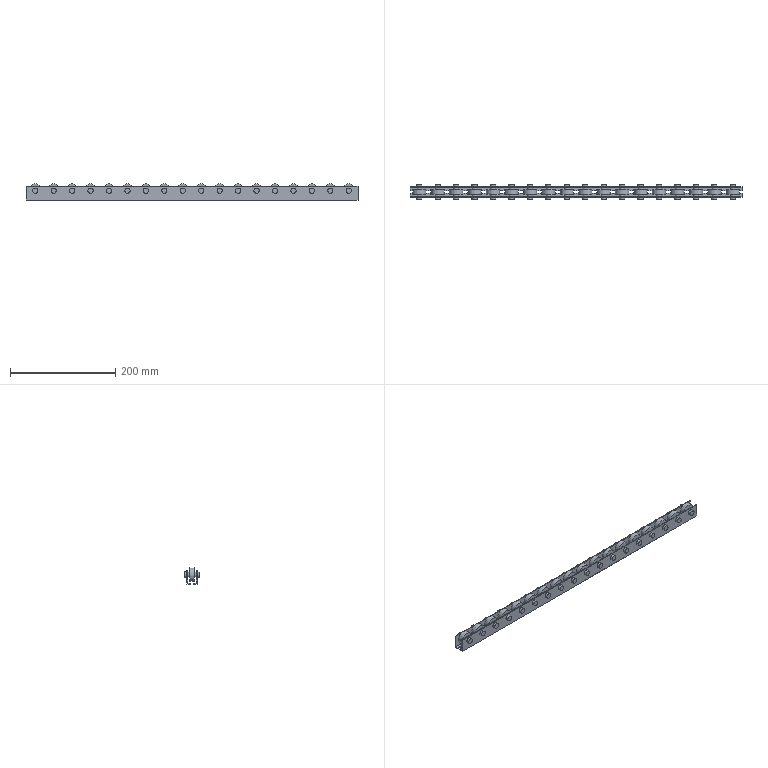Part | NX | features solid 2 | 1 solid | 178 faces | box 630 x 29 x 30.5 mm | volume 169139 mm3 | cylinder 90 | plane 88 | commonest cylinder face diameters 10 x72 25.4 x18